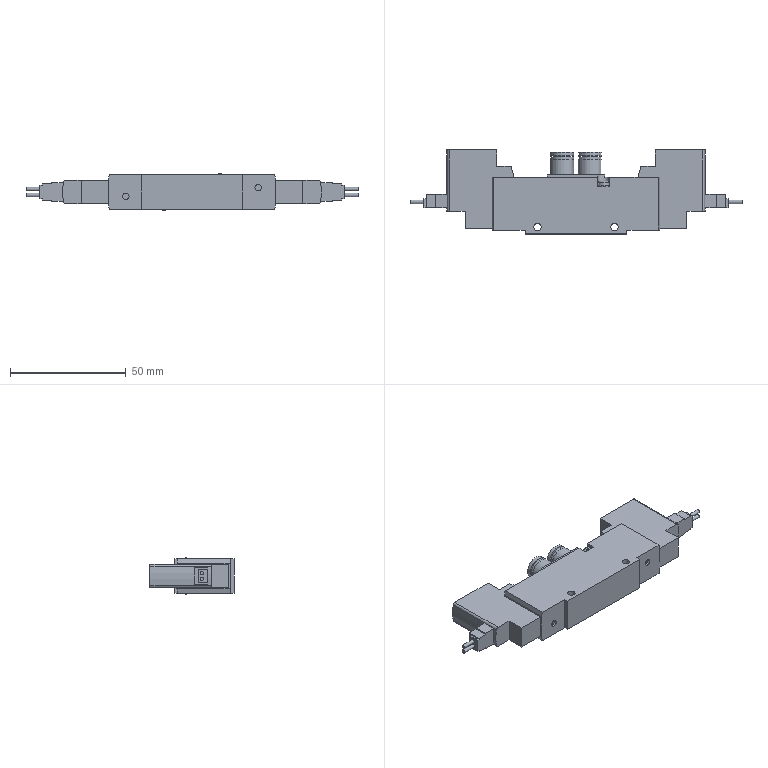Part | NX | 1 solid | 128 faces | box 143.4 x 36.3 x 15.8 mm | volume 40855 mm3 | plane 94 | cylinder 32 | spline 2 | commonest cylinder face diameters 1.5 x4 2 x4 9.9 x4 2.8 x2 3.2 x2 3.3 x2